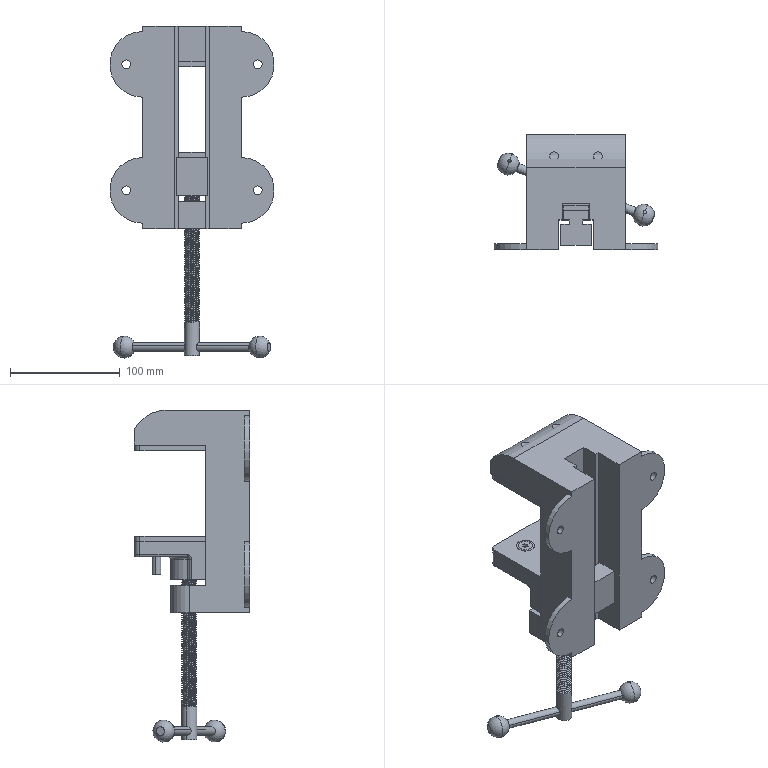Part | SolidWorks | features MirrorCompFeat 2, CompositeCurve 1, ReferencePattern 1 | 14 solids | 459 faces | box 150 x 105 x 303.032 mm | volume 931292 mm3 | cylinder 243 | plane 146 | cone 42 | torus 13 | spline 9 | sphere 6 | commonest cylinder face diameters 13.8 x116 12 x26 8 x24 3 x14 9.8 x13 4 x9